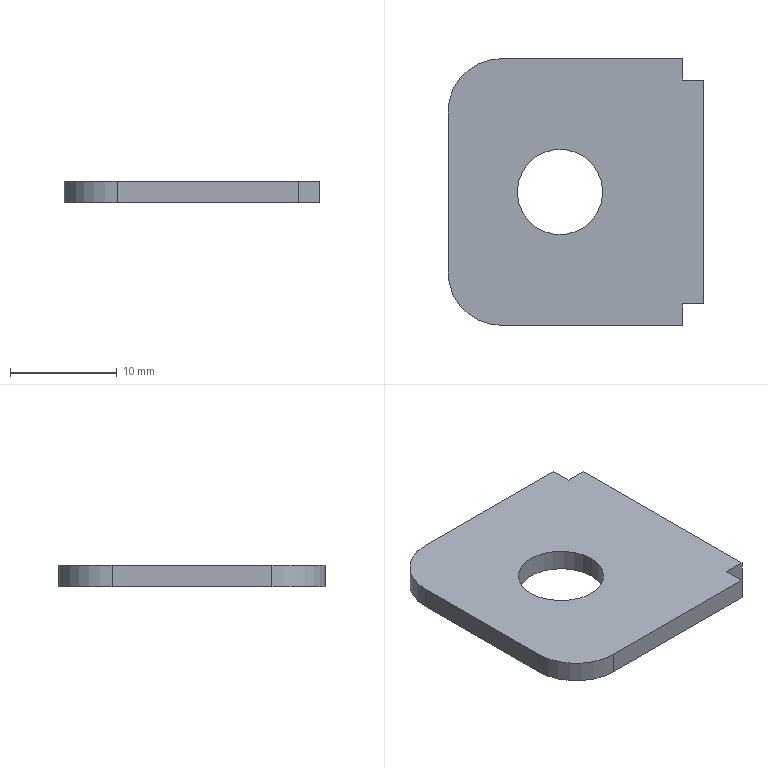Part | STEP file | SYL_0392D6J1SYL0380DJ100-884005 | 1 solid | 14 faces | box 24 x 25 x 2 mm | volume 1062 mm3 | plane 10 | cylinder 4 | commonest cylinder face diameters 8 x2 10 x2
STEP:
#1=CARTESIAN_POINT('',(-5.5,0.,0.));
#2=VERTEX_POINT('',#1);
#3=CARTESIAN_POINT('',(2.5,0.,0.));
#4=VERTEX_POINT('',#3);
#5=CARTESIAN_POINT('',(-1.5,0.,0.));
#6=DIRECTION('',(0.,0.,-1.));
#7=DIRECTION('',(-1.,0.,0.));
#8=AXIS2_PLACEMENT_3D('',#5,#6,#7);
#9=CIRCLE('',#8,4.);
#10=EDGE_CURVE('',#2,#4,#9,.T.);
#11=ORIENTED_EDGE('',*,*,#10,.F.);
#12=CARTESIAN_POINT('',(-5.5,0.,-2.));
#13=VERTEX_POINT('',#12);
#14=CARTESIAN_POINT('',(-5.5,0.,-2.));
#15=DIRECTION('',(0.,0.,1.));
#16=VECTOR('',#15,1000.);
#17=LINE('',#14,#16);
#18=EDGE_CURVE('',#13,#2,#17,.T.);
#19=ORIENTED_EDGE('',*,*,#18,.F.);
#20=CARTESIAN_POINT('',(2.5,0.,-2.));
#21=VERTEX_POINT('',#20);
#22=CARTESIAN_POINT('',(-1.5,0.,-2.));
#23=DIRECTION('',(0.,0.,1.));
#24=DIRECTION('',(1.,0.,0.));
#25=AXIS2_PLACEMENT_3D('',#22,#23,#24);
#26=CIRCLE('',#25,4.);
#27=EDGE_CURVE('',#21,#13,#26,.T.);
#28=ORIENTED_EDGE('',*,*,#27,.F.);
#29=CARTESIAN_POINT('',(2.5,0.,-2.));
#30=DIRECTION('',(0.,0.,1.));
#31=VECTOR('',#30,1000.);
#32=LINE('',#29,#31);
#33=EDGE_CURVE('',#21,#4,#32,.T.);
#34=ORIENTED_EDGE('',*,*,#33,.T.);
#35=EDGE_LOOP('',(#11,#19,#28,#34));
#36=FACE_OUTER_BOUND('',#35,.T.);
#37=CARTESIAN_POINT('',(-1.5,0.,-1.));
#38=DIRECTION('',(0.,0.,-1.));
#39=DIRECTION('',(-1.,0.,0.));
#40=AXIS2_PLACEMENT_3D('',#37,#38,#39);
#41=CYLINDRICAL_SURFACE('',#40,4.);
#42=ADVANCED_FACE('',(#36),#41,.F.);
#43=CARTESIAN_POINT('',(10.,10.5,0.));
#44=VERTEX_POINT('',#43);
#45=CARTESIAN_POINT('',(12.,10.5,0.));
#46=VERTEX_POINT('',#45);
#47=CARTESIAN_POINT('',(10.,10.5,0.));
#48=DIRECTION('',(1.,0.,0.));
#49=VECTOR('',#48,1000.);
#50=LINE('',#47,#49);
#51=EDGE_CURVE('',#44,#46,#50,.T.);
#52=ORIENTED_EDGE('',*,*,#51,.T.);
#53=CARTESIAN_POINT('',(12.,10.5,-2.));
#54=VERTEX_POINT('',#53);
#55=CARTESIAN_POINT('',(12.,10.5,-2.));
#56=DIRECTION('',(0.,0.,1.));
#57=VECTOR('',#56,1000.);
#58=LINE('',#55,#57);
#59=EDGE_CURVE('',#54,#46,#58,.T.);
#60=ORIENTED_EDGE('',*,*,#59,.F.);
#61=CARTESIAN_POINT('',(10.,10.5,-2.));
#62=VERTEX_POINT('',#61);
#63=CARTESIAN_POINT('',(10.,10.5,-2.));
#64=DIRECTION('',(1.,0.,0.));
#65=VECTOR('',#64,1000.);
#66=LINE('',#63,#65);
#67=EDGE_CURVE('',#62,#54,#66,.T.);
#68=ORIENTED_EDGE('',*,*,#67,.F.);
#69=CARTESIAN_POINT('',(10.,10.5,0.));
#70=DIRECTION('',(0.,0.,-1.));
#71=VECTOR('',#70,1000.);
#72=LINE('',#69,#71);
#73=EDGE_CURVE('',#44,#62,#72,.T.);
#74=ORIENTED_EDGE('',*,*,#73,.F.);
#75=EDGE_LOOP('',(#52,#60,#68,#74));
#76=FACE_OUTER_BOUND('',#75,.T.);
#77=CARTESIAN_POINT('',(11.,10.5,-1.));
#78=DIRECTION('',(0.,1.,0.));
#79=DIRECTION('',(1.,0.,0.));
#80=AXIS2_PLACEMENT_3D('',#77,#78,#79);
#81=PLANE('',#80);
#82=ADVANCED_FACE('',(#76),#81,.T.);
#83=CARTESIAN_POINT('',(10.,12.5,-2.));
#84=VERTEX_POINT('',#83);
#85=CARTESIAN_POINT('',(10.,12.5,0.));
#86=VERTEX_POINT('',#85);
#87=CARTESIAN_POINT('',(10.,12.5,-2.));
#88=DIRECTION('',(0.,0.,1.));
#89=VECTOR('',#88,1000.);
#90=LINE('',#87,#89);
#91=EDGE_CURVE('',#84,#86,#90,.T.);
#92=ORIENTED_EDGE('',*,*,#91,.T.);
#93=CARTESIAN_POINT('',(10.,12.5,0.));
#94=DIRECTION('',(0.,-1.,0.));
#95=VECTOR('',#94,1000.);
#96=LINE('',#93,#95);
#97=EDGE_CURVE('',#86,#44,#96,.T.);
#98=ORIENTED_EDGE('',*,*,#97,.T.);
#99=ORIENTED_EDGE('',*,*,#73,.T.);
#100=CARTESIAN_POINT('',(10.,10.5,-2.));
#101=DIRECTION('',(0.,1.,0.));
#102=VECTOR('',#101,1000.);
#103=LINE('',#100,#102);
#104=EDGE_CURVE('',#62,#84,#103,.T.);
#105=ORIENTED_EDGE('',*,*,#104,.T.);
#106=EDGE_LOOP('',(#92,#98,#99,#105));
#107=FACE_OUTER_BOUND('',#106,.T.);
#108=CARTESIAN_POINT('',(10.,11.5,-1.));
#109=DIRECTION('',(-1.,0.,0.));
#110=DIRECTION('',(0.,0.,1.));
#111=AXIS2_PLACEMENT_3D('',#108,#109,#110);
#112=PLANE('',#111);
#113=ADVANCED_FACE('',(#107),#112,.F.);
#114=ORIENTED_EDGE('',*,*,#91,.F.);
#115=CARTESIAN_POINT('',(-7.,12.5,-2.));
#116=VERTEX_POINT('',#115);
#117=CARTESIAN_POINT('',(-7.,12.5,-2.));
#118=DIRECTION('',(1.,0.,0.));
#119=VECTOR('',#118,1000.);
#120=LINE('',#117,#119);
#121=EDGE_CURVE('',#116,#84,#120,.T.);
#122=ORIENTED_EDGE('',*,*,#121,.F.);
#123=CARTESIAN_POINT('',(-7.,12.5,0.));
#124=VERTEX_POINT('',#123);
#125=CARTESIAN_POINT('',(-7.,12.5,0.));
#126=DIRECTION('',(0.,0.,-1.));
#127=VECTOR('',#126,1000.);
#128=LINE('',#125,#127);
#129=EDGE_CURVE('',#124,#116,#128,.T.);
#130=ORIENTED_EDGE('',*,*,#129,.F.);
#131=CARTESIAN_POINT('',(-7.,12.5,0.));
#132=DIRECTION('',(1.,0.,0.));
#133=VECTOR('',#132,1000.);
#134=LINE('',#131,#133);
#135=EDGE_CURVE('',#124,#86,#134,.T.);
#136=ORIENTED_EDGE('',*,*,#135,.T.);
#137=EDGE_LOOP('',(#114,#122,#130,#136));
#138=FACE_OUTER_BOUND('',#137,.T.);
#139=CARTESIAN_POINT('',(2.5,12.5,-1.));
#140=DIRECTION('',(0.,1.,0.));
#141=DIRECTION('',(1.,0.,0.));
#142=AXIS2_PLACEMENT_3D('',#139,#140,#141);
#143=PLANE('',#142);
#144=ADVANCED_FACE('',(#138),#143,.T.);
#145=CARTESIAN_POINT('',(-12.,7.5,0.));
#146=VERTEX_POINT('',#145);
#147=CARTESIAN_POINT('',(-7.,7.5,0.));
#148=DIRECTION('',(0.,0.,1.));
#149=DIRECTION('',(0.,1.,0.));
#150=AXIS2_PLACEMENT_3D('',#147,#148,#149);
#151=CIRCLE('',#150,5.);
#152=EDGE_CURVE('',#124,#146,#151,.T.);
#153=ORIENTED_EDGE('',*,*,#152,.F.);
#154=ORIENTED_EDGE('',*,*,#129,.T.);
#155=CARTESIAN_POINT('',(-12.,7.5,-2.));
#156=VERTEX_POINT('',#155);
#157=CARTESIAN_POINT('',(-7.,7.5,-2.));
#158=DIRECTION('',(0.,0.,-1.));
#159=DIRECTION('',(-1.,0.,0.));
#160=AXIS2_PLACEMENT_3D('',#157,#158,#159);
#161=CIRCLE('',#160,5.);
#162=EDGE_CURVE('',#156,#116,#161,.T.);
#163=ORIENTED_EDGE('',*,*,#162,.F.);
#164=CARTESIAN_POINT('',(-12.,7.5,-2.));
#165=DIRECTION('',(0.,0.,1.));
#166=VECTOR('',#165,1000.);
#167=LINE('',#164,#166);
#168=EDGE_CURVE('',#156,#146,#167,.T.);
#169=ORIENTED_EDGE('',*,*,#168,.T.);
#170=EDGE_LOOP('',(#153,#154,#163,#169));
#171=FACE_OUTER_BOUND('',#170,.T.);
#172=CARTESIAN_POINT('',(-7.,7.5,-1.));
#173=DIRECTION('',(0.,0.,1.));
#174=DIRECTION('',(1.,0.,0.));
#175=AXIS2_PLACEMENT_3D('',#172,#173,#174);
#176=CYLINDRICAL_SURFACE('',#175,5.);
#177=ADVANCED_FACE('',(#171),#176,.T.);
#178=CARTESIAN_POINT('',(-12.,-7.5,0.));
#179=VERTEX_POINT('',#178);
#180=CARTESIAN_POINT('',(-12.,-7.5,0.));
#181=DIRECTION('',(0.,1.,0.));
#182=VECTOR('',#181,1000.);
#183=LINE('',#180,#182);
#184=EDGE_CURVE('',#179,#146,#183,.T.);
#185=ORIENTED_EDGE('',*,*,#184,.T.);
#186=ORIENTED_EDGE('',*,*,#168,.F.);
#187=CARTESIAN_POINT('',(-12.,-7.5,-2.));
#188=VERTEX_POINT('',#187);
#189=CARTESIAN_POINT('',(-12.,-7.5,-2.));
#190=DIRECTION('',(0.,1.,0.));
#191=VECTOR('',#190,1000.);
#192=LINE('',#189,#191);
#193=EDGE_CURVE('',#188,#156,#192,.T.);
#194=ORIENTED_EDGE('',*,*,#193,.F.);
#195=CARTESIAN_POINT('',(-12.,-7.5,0.));
#196=DIRECTION('',(0.,0.,-1.));
#197=VECTOR('',#196,1000.);
#198=LINE('',#195,#197);
#199=EDGE_CURVE('',#179,#188,#198,.T.);
#200=ORIENTED_EDGE('',*,*,#199,.F.);
#201=EDGE_LOOP('',(#185,#186,#194,#200));
#202=FACE_OUTER_BOUND('',#201,.T.);
#203=CARTESIAN_POINT('',(-12.,0.,-1.));
#204=DIRECTION('',(-1.,0.,0.));
#205=DIRECTION('',(0.,0.,1.));
#206=AXIS2_PLACEMENT_3D('',#203,#204,#205);
#207=PLANE('',#206);
#208=ADVANCED_FACE('',(#202),#207,.T.);
#209=CARTESIAN_POINT('',(-7.,-12.5,0.));
#210=VERTEX_POINT('',#209);
#211=CARTESIAN_POINT('',(-7.,-7.5,0.));
#212=DIRECTION('',(0.,0.,1.));
#213=DIRECTION('',(-1.,0.,0.));
#214=AXIS2_PLACEMENT_3D('',#211,#212,#213);
#215=CIRCLE('',#214,5.);
#216=EDGE_CURVE('',#179,#210,#215,.T.);
#217=ORIENTED_EDGE('',*,*,#216,.F.);
#218=ORIENTED_EDGE('',*,*,#199,.T.);
#219=CARTESIAN_POINT('',(-7.,-12.5,-2.));
#220=VERTEX_POINT('',#219);
#221=CARTESIAN_POINT('',(-7.,-7.5,-2.));
#222=DIRECTION('',(0.,0.,-1.));
#223=DIRECTION('',(0.,-1.,0.));
#224=AXIS2_PLACEMENT_3D('',#221,#222,#223);
#225=CIRCLE('',#224,5.);
#226=EDGE_CURVE('',#220,#188,#225,.T.);
#227=ORIENTED_EDGE('',*,*,#226,.F.);
#228=CARTESIAN_POINT('',(-7.,-12.5,-2.));
#229=DIRECTION('',(0.,0.,1.));
#230=VECTOR('',#229,1000.);
#231=LINE('',#228,#230);
#232=EDGE_CURVE('',#220,#210,#231,.T.);
#233=ORIENTED_EDGE('',*,*,#232,.T.);
#234=EDGE_LOOP('',(#217,#218,#227,#233));
#235=FACE_OUTER_BOUND('',#234,.T.);
#236=CARTESIAN_POINT('',(-7.,-7.5,-1.));
#237=DIRECTION('',(0.,0.,1.));
#238=DIRECTION('',(1.,0.,0.));
#239=AXIS2_PLACEMENT_3D('',#236,#237,#238);
#240=CYLINDRICAL_SURFACE('',#239,5.);
#241=ADVANCED_FACE('',(#235),#240,.T.);
#242=CARTESIAN_POINT('',(10.,-12.5,-2.));
#243=VERTEX_POINT('',#242);
#244=CARTESIAN_POINT('',(10.,-12.5,0.));
#245=VERTEX_POINT('',#244);
#246=CARTESIAN_POINT('',(10.,-12.5,-2.));
#247=DIRECTION('',(0.,0.,1.));
#248=VECTOR('',#247,1000.);
#249=LINE('',#246,#248);
#250=EDGE_CURVE('',#243,#245,#249,.T.);
#251=ORIENTED_EDGE('',*,*,#250,.T.);
#252=CARTESIAN_POINT('',(10.,-12.5,0.));
#253=DIRECTION('',(-1.,0.,0.));
#254=VECTOR('',#253,1000.);
#255=LINE('',#252,#254);
#256=EDGE_CURVE('',#245,#210,#255,.T.);
#257=ORIENTED_EDGE('',*,*,#256,.T.);
#258=ORIENTED_EDGE('',*,*,#232,.F.);
#259=CARTESIAN_POINT('',(10.,-12.5,-2.));
#260=DIRECTION('',(-1.,0.,0.));
#261=VECTOR('',#260,1000.);
#262=LINE('',#259,#261);
#263=EDGE_CURVE('',#243,#220,#262,.T.);
#264=ORIENTED_EDGE('',*,*,#263,.F.);
#265=EDGE_LOOP('',(#251,#257,#258,#264));
#266=FACE_OUTER_BOUND('',#265,.T.);
#267=CARTESIAN_POINT('',(2.5,-12.5,-1.));
#268=DIRECTION('',(0.,-1.,0.));
#269=DIRECTION('',(0.,0.,-1.));
#270=AXIS2_PLACEMENT_3D('',#267,#268,#269);
#271=PLANE('',#270);
#272=ADVANCED_FACE('',(#266),#271,.T.);
#273=CARTESIAN_POINT('',(10.,-10.5,0.));
#274=VERTEX_POINT('',#273);
#275=CARTESIAN_POINT('',(10.,-10.5,0.));
#276=DIRECTION('',(0.,-1.,0.));
#277=VECTOR('',#276,1000.);
#278=LINE('',#275,#277);
#279=EDGE_CURVE('',#274,#245,#278,.T.);
#280=ORIENTED_EDGE('',*,*,#279,.T.);
#281=ORIENTED_EDGE('',*,*,#250,.F.);
#282=CARTESIAN_POINT('',(10.,-10.5,-2.));
#283=VERTEX_POINT('',#282);
#284=CARTESIAN_POINT('',(10.,-10.5,-2.));
#285=DIRECTION('',(0.,-1.,0.));
#286=VECTOR('',#285,1000.);
#287=LINE('',#284,#286);
#288=EDGE_CURVE('',#283,#243,#287,.T.);
#289=ORIENTED_EDGE('',*,*,#288,.F.);
#290=CARTESIAN_POINT('',(10.,-10.5,0.));
#291=DIRECTION('',(0.,0.,-1.));
#292=VECTOR('',#291,1000.);
#293=LINE('',#290,#292);
#294=EDGE_CURVE('',#274,#283,#293,.T.);
#295=ORIENTED_EDGE('',*,*,#294,.F.);
#296=EDGE_LOOP('',(#280,#281,#289,#295));
#297=FACE_OUTER_BOUND('',#296,.T.);
#298=CARTESIAN_POINT('',(10.,-11.5,-1.));
#299=DIRECTION('',(1.,0.,0.));
#300=DIRECTION('',(0.,1.,0.));
#301=AXIS2_PLACEMENT_3D('',#298,#299,#300);
#302=PLANE('',#301);
#303=ADVANCED_FACE('',(#297),#302,.T.);
#304=CARTESIAN_POINT('',(12.,-10.5,-2.));
#305=VERTEX_POINT('',#304);
#306=CARTESIAN_POINT('',(12.,-10.5,0.));
#307=VERTEX_POINT('',#306);
#308=CARTESIAN_POINT('',(12.,-10.5,-2.));
#309=DIRECTION('',(0.,0.,1.));
#310=VECTOR('',#309,1000.);
#311=LINE('',#308,#310);
#312=EDGE_CURVE('',#305,#307,#311,.T.);
#313=ORIENTED_EDGE('',*,*,#312,.T.);
#314=CARTESIAN_POINT('',(12.,-10.5,0.));
#315=DIRECTION('',(-1.,0.,0.));
#316=VECTOR('',#315,1000.);
#317=LINE('',#314,#316);
#318=EDGE_CURVE('',#307,#274,#317,.T.);
#319=ORIENTED_EDGE('',*,*,#318,.T.);
#320=ORIENTED_EDGE('',*,*,#294,.T.);
#321=CARTESIAN_POINT('',(10.,-10.5,-2.));
#322=DIRECTION('',(1.,0.,0.));
#323=VECTOR('',#322,1000.);
#324=LINE('',#321,#323);
#325=EDGE_CURVE('',#283,#305,#324,.T.);
#326=ORIENTED_EDGE('',*,*,#325,.T.);
#327=EDGE_LOOP('',(#313,#319,#320,#326));
#328=FACE_OUTER_BOUND('',#327,.T.);
#329=CARTESIAN_POINT('',(11.,-10.5,-1.));
#330=DIRECTION('',(0.,1.,0.));
#331=DIRECTION('',(1.,0.,0.));
#332=AXIS2_PLACEMENT_3D('',#329,#330,#331);
#333=PLANE('',#332);
#334=ADVANCED_FACE('',(#328),#333,.F.);
#335=ORIENTED_EDGE('',*,*,#27,.T.);
#336=CARTESIAN_POINT('',(-1.5,0.,-2.));
#337=DIRECTION('',(0.,0.,1.));
#338=DIRECTION('',(-1.,0.,0.));
#339=AXIS2_PLACEMENT_3D('',#336,#337,#338);
#340=CIRCLE('',#339,4.);
#341=EDGE_CURVE('',#13,#21,#340,.T.);
#342=ORIENTED_EDGE('',*,*,#341,.T.);
#343=EDGE_LOOP('',(#335,#342));
#344=FACE_BOUND('',#343,.T.);
#345=ORIENTED_EDGE('',*,*,#288,.T.);
#346=ORIENTED_EDGE('',*,*,#263,.T.);
#347=ORIENTED_EDGE('',*,*,#226,.T.);
#348=ORIENTED_EDGE('',*,*,#193,.T.);
#349=ORIENTED_EDGE('',*,*,#162,.T.);
#350=ORIENTED_EDGE('',*,*,#121,.T.);
#351=ORIENTED_EDGE('',*,*,#104,.F.);
#352=ORIENTED_EDGE('',*,*,#67,.T.);
#353=CARTESIAN_POINT('',(12.,10.5,-2.));
#354=DIRECTION('',(0.,-1.,0.));
#355=VECTOR('',#354,1000.);
#356=LINE('',#353,#355);
#357=EDGE_CURVE('',#54,#305,#356,.T.);
#358=ORIENTED_EDGE('',*,*,#357,.T.);
#359=ORIENTED_EDGE('',*,*,#325,.F.);
#360=EDGE_LOOP('',(#345,#346,#347,#348,#349,#350,#351,#352,#358,#359));
#361=FACE_OUTER_BOUND('',#360,.T.);
#362=CARTESIAN_POINT('',(0.,0.,-2.));
#363=DIRECTION('',(0.,0.,1.));
#364=DIRECTION('',(1.,0.,0.));
#365=AXIS2_PLACEMENT_3D('',#362,#363,#364);
#366=PLANE('',#365);
#367=ADVANCED_FACE('',(#344,#361),#366,.F.);
#368=ORIENTED_EDGE('',*,*,#59,.T.);
#369=CARTESIAN_POINT('',(12.,10.5,0.));
#370=DIRECTION('',(0.,-1.,0.));
#371=VECTOR('',#370,1000.);
#372=LINE('',#369,#371);
#373=EDGE_CURVE('',#46,#307,#372,.T.);
#374=ORIENTED_EDGE('',*,*,#373,.T.);
#375=ORIENTED_EDGE('',*,*,#312,.F.);
#376=ORIENTED_EDGE('',*,*,#357,.F.);
#377=EDGE_LOOP('',(#368,#374,#375,#376));
#378=FACE_OUTER_BOUND('',#377,.T.);
#379=CARTESIAN_POINT('',(12.,0.,-1.));
#380=DIRECTION('',(1.,0.,0.));
#381=DIRECTION('',(0.,1.,0.));
#382=AXIS2_PLACEMENT_3D('',#379,#380,#381);
#383=PLANE('',#382);
#384=ADVANCED_FACE('',(#378),#383,.T.);
#385=CARTESIAN_POINT('',(-1.5,0.,0.));
#386=DIRECTION('',(0.,0.,-1.));
#387=DIRECTION('',(1.,0.,0.));
#388=AXIS2_PLACEMENT_3D('',#385,#386,#387);
#389=CIRCLE('',#388,4.);
#390=EDGE_CURVE('',#4,#2,#389,.T.);
#391=ORIENTED_EDGE('',*,*,#390,.T.);
#392=ORIENTED_EDGE('',*,*,#10,.T.);
#393=EDGE_LOOP('',(#391,#392));
#394=FACE_BOUND('',#393,.T.);
#395=ORIENTED_EDGE('',*,*,#51,.F.);
#396=ORIENTED_EDGE('',*,*,#97,.F.);
#397=ORIENTED_EDGE('',*,*,#135,.F.);
#398=ORIENTED_EDGE('',*,*,#152,.T.);
#399=ORIENTED_EDGE('',*,*,#184,.F.);
#400=ORIENTED_EDGE('',*,*,#216,.T.);
#401=ORIENTED_EDGE('',*,*,#256,.F.);
#402=ORIENTED_EDGE('',*,*,#279,.F.);
#403=ORIENTED_EDGE('',*,*,#318,.F.);
#404=ORIENTED_EDGE('',*,*,#373,.F.);
#405=EDGE_LOOP('',(#395,#396,#397,#398,#399,#400,#401,#402,#403,#404));
#406=FACE_OUTER_BOUND('',#405,.T.);
#407=CARTESIAN_POINT('',(0.,0.,0.));
#408=DIRECTION('',(0.,0.,1.));
#409=DIRECTION('',(1.,0.,0.));
#410=AXIS2_PLACEMENT_3D('',#407,#408,#409);
#411=PLANE('',#410);
#412=ADVANCED_FACE('',(#394,#406),#411,.T.);
#413=ORIENTED_EDGE('',*,*,#33,.F.);
#414=ORIENTED_EDGE('',*,*,#341,.F.);
#415=ORIENTED_EDGE('',*,*,#18,.T.);
#416=ORIENTED_EDGE('',*,*,#390,.F.);
#417=EDGE_LOOP('',(#413,#414,#415,#416));
#418=FACE_OUTER_BOUND('',#417,.T.);
#419=CARTESIAN_POINT('',(-1.5,0.,-1.));
#420=DIRECTION('',(0.,0.,-1.));
#421=DIRECTION('',(-1.,0.,0.));
#422=AXIS2_PLACEMENT_3D('',#419,#420,#421);
#423=CYLINDRICAL_SURFACE('',#422,4.);
#424=ADVANCED_FACE('',(#418),#423,.F.);
#425=CLOSED_SHELL('',(#42,#82,#113,#144,#177,#208,#241,#272,#303,#334,#367,#384,#412,#424));
#426=MANIFOLD_SOLID_BREP('',#425);
#427=CARTESIAN_POINT('',(0.,0.,0.));
#428=DIRECTION('',(0.,0.,1.));
#429=DIRECTION('',(1.,0.,0.));
#430=AXIS2_PLACEMENT_3D('',#427,#428,#429);
#431=(LENGTH_UNIT()NAMED_UNIT(*)SI_UNIT(.MILLI.,.METRE.));
#432=UNCERTAINTY_MEASURE_WITH_UNIT(LENGTH_MEASURE(0.00001),#431,'','');
#433=(NAMED_UNIT(*)PLANE_ANGLE_UNIT()SI_UNIT($,.RADIAN.));
#434=(NAMED_UNIT(*)SI_UNIT($,.STERADIAN.)SOLID_ANGLE_UNIT());
#435=(GEOMETRIC_REPRESENTATION_CONTEXT(3)GLOBAL_UNCERTAINTY_ASSIGNED_CONTEXT((#432))GLOBAL_UNIT_ASSIGNED_CONTEXT((#431,#433,#434))REPRESENTATION_CONTEXT('',''));
#436=ADVANCED_BREP_SHAPE_REPRESENTATION('',(#426,#430),#435);